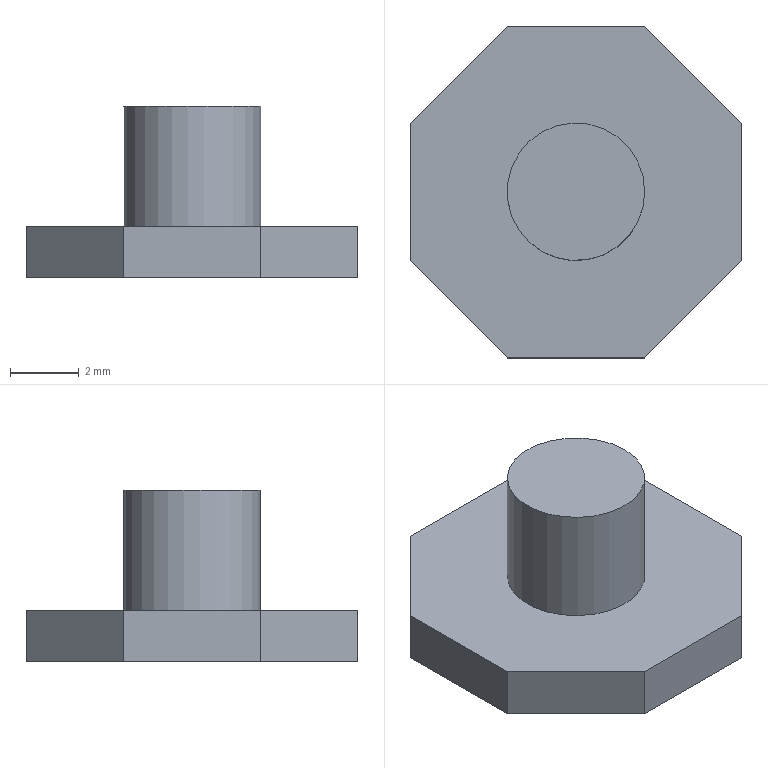Part | NX | features DATUM_CSYS 2, EXTRUDE 2, SKETCH 1 | 1 solid | 12 faces | box 9.657 x 9.657 x 5 mm | volume 159.865 mm3 | plane 11 | cylinder 1 | commonest cylinder face diameters 4 x1
STEP:
#1=CARTESIAN_POINT('',(-4.828,2.,0.));
#2=VERTEX_POINT('',#1);
#3=CARTESIAN_POINT('',(-4.828,-2.,0.));
#4=VERTEX_POINT('',#3);
#5=CARTESIAN_POINT('',(-4.828,2.,0.));
#6=DIRECTION('',(0.,-1.,0.));
#7=VECTOR('',#6,1000.);
#8=LINE('',#5,#7);
#9=EDGE_CURVE('',#2,#4,#8,.T.);
#10=ORIENTED_EDGE('',*,*,#9,.T.);
#11=CARTESIAN_POINT('',(-4.828,-2.,1.5));
#12=VERTEX_POINT('',#11);
#13=CARTESIAN_POINT('',(-4.828,-2.,1.5));
#14=DIRECTION('',(0.,0.,-1.));
#15=VECTOR('',#14,1000.);
#16=LINE('',#13,#15);
#17=EDGE_CURVE('',#12,#4,#16,.T.);
#18=ORIENTED_EDGE('',*,*,#17,.F.);
#19=CARTESIAN_POINT('',(-4.828,2.,1.5));
#20=VERTEX_POINT('',#19);
#21=CARTESIAN_POINT('',(-4.828,2.,1.5));
#22=DIRECTION('',(0.,-1.,0.));
#23=VECTOR('',#22,1000.);
#24=LINE('',#21,#23);
#25=EDGE_CURVE('',#20,#12,#24,.T.);
#26=ORIENTED_EDGE('',*,*,#25,.F.);
#27=CARTESIAN_POINT('',(-4.828,2.,1.5));
#28=DIRECTION('',(0.,0.,-1.));
#29=VECTOR('',#28,1000.);
#30=LINE('',#27,#29);
#31=EDGE_CURVE('',#20,#2,#30,.T.);
#32=ORIENTED_EDGE('',*,*,#31,.T.);
#33=EDGE_LOOP('',(#10,#18,#26,#32));
#34=FACE_BOUND('',#33,.T.);
#35=CARTESIAN_POINT('',(-4.828,2.,1.5));
#36=DIRECTION('',(1.,0.,0.));
#37=DIRECTION('',(0.,0.,-1.));
#38=AXIS2_PLACEMENT_3D('',#35,#36,#37);
#39=PLANE('',#38);
#40=ADVANCED_FACE('',(#34),#39,.F.);
#41=CARTESIAN_POINT('',(-2.,-4.828,0.));
#42=VERTEX_POINT('',#41);
#43=CARTESIAN_POINT('',(-4.828,-2.,0.));
#44=DIRECTION('',(0.7071,-0.7071,0.));
#45=VECTOR('',#44,1000.);
#46=LINE('',#43,#45);
#47=EDGE_CURVE('',#4,#42,#46,.T.);
#48=ORIENTED_EDGE('',*,*,#47,.T.);
#49=CARTESIAN_POINT('',(-2.,-4.828,1.5));
#50=VERTEX_POINT('',#49);
#51=CARTESIAN_POINT('',(-2.,-4.828,1.5));
#52=DIRECTION('',(0.,0.,-1.));
#53=VECTOR('',#52,1000.);
#54=LINE('',#51,#53);
#55=EDGE_CURVE('',#50,#42,#54,.T.);
#56=ORIENTED_EDGE('',*,*,#55,.F.);
#57=CARTESIAN_POINT('',(-4.828,-2.,1.5));
#58=DIRECTION('',(0.7071,-0.7071,0.));
#59=VECTOR('',#58,1000.);
#60=LINE('',#57,#59);
#61=EDGE_CURVE('',#12,#50,#60,.T.);
#62=ORIENTED_EDGE('',*,*,#61,.F.);
#63=ORIENTED_EDGE('',*,*,#17,.T.);
#64=EDGE_LOOP('',(#48,#56,#62,#63));
#65=FACE_BOUND('',#64,.T.);
#66=CARTESIAN_POINT('',(-4.828,-2.,1.5));
#67=DIRECTION('',(0.7071,0.7071,0.));
#68=DIRECTION('',(-0.7071,0.7071,0.));
#69=AXIS2_PLACEMENT_3D('',#66,#67,#68);
#70=PLANE('',#69);
#71=ADVANCED_FACE('',(#65),#70,.F.);
#72=CARTESIAN_POINT('',(2.,-4.828,0.));
#73=VERTEX_POINT('',#72);
#74=CARTESIAN_POINT('',(-2.,-4.828,0.));
#75=DIRECTION('',(1.,0.,0.));
#76=VECTOR('',#75,1000.);
#77=LINE('',#74,#76);
#78=EDGE_CURVE('',#42,#73,#77,.T.);
#79=ORIENTED_EDGE('',*,*,#78,.T.);
#80=CARTESIAN_POINT('',(2.,-4.828,1.5));
#81=VERTEX_POINT('',#80);
#82=CARTESIAN_POINT('',(2.,-4.828,1.5));
#83=DIRECTION('',(0.,0.,-1.));
#84=VECTOR('',#83,1000.);
#85=LINE('',#82,#84);
#86=EDGE_CURVE('',#81,#73,#85,.T.);
#87=ORIENTED_EDGE('',*,*,#86,.F.);
#88=CARTESIAN_POINT('',(-2.,-4.828,1.5));
#89=DIRECTION('',(1.,0.,0.));
#90=VECTOR('',#89,1000.);
#91=LINE('',#88,#90);
#92=EDGE_CURVE('',#50,#81,#91,.T.);
#93=ORIENTED_EDGE('',*,*,#92,.F.);
#94=ORIENTED_EDGE('',*,*,#55,.T.);
#95=EDGE_LOOP('',(#79,#87,#93,#94));
#96=FACE_BOUND('',#95,.T.);
#97=CARTESIAN_POINT('',(-2.,-4.828,1.5));
#98=DIRECTION('',(0.,1.,0.));
#99=DIRECTION('',(-1.,0.,0.));
#100=AXIS2_PLACEMENT_3D('',#97,#98,#99);
#101=PLANE('',#100);
#102=ADVANCED_FACE('',(#96),#101,.F.);
#103=CARTESIAN_POINT('',(4.828,-2.,0.));
#104=VERTEX_POINT('',#103);
#105=CARTESIAN_POINT('',(2.,-4.828,0.));
#106=DIRECTION('',(0.7071,0.7071,0.));
#107=VECTOR('',#106,1000.);
#108=LINE('',#105,#107);
#109=EDGE_CURVE('',#73,#104,#108,.T.);
#110=ORIENTED_EDGE('',*,*,#109,.T.);
#111=CARTESIAN_POINT('',(4.828,-2.,1.5));
#112=VERTEX_POINT('',#111);
#113=CARTESIAN_POINT('',(4.828,-2.,1.5));
#114=DIRECTION('',(0.,0.,-1.));
#115=VECTOR('',#114,1000.);
#116=LINE('',#113,#115);
#117=EDGE_CURVE('',#112,#104,#116,.T.);
#118=ORIENTED_EDGE('',*,*,#117,.F.);
#119=CARTESIAN_POINT('',(2.,-4.828,1.5));
#120=DIRECTION('',(0.7071,0.7071,0.));
#121=VECTOR('',#120,1000.);
#122=LINE('',#119,#121);
#123=EDGE_CURVE('',#81,#112,#122,.T.);
#124=ORIENTED_EDGE('',*,*,#123,.F.);
#125=ORIENTED_EDGE('',*,*,#86,.T.);
#126=EDGE_LOOP('',(#110,#118,#124,#125));
#127=FACE_BOUND('',#126,.T.);
#128=CARTESIAN_POINT('',(2.,-4.828,1.5));
#129=DIRECTION('',(-0.7071,0.7071,0.));
#130=DIRECTION('',(-0.7071,-0.7071,0.));
#131=AXIS2_PLACEMENT_3D('',#128,#129,#130);
#132=PLANE('',#131);
#133=ADVANCED_FACE('',(#127),#132,.F.);
#134=CARTESIAN_POINT('',(4.828,2.,0.));
#135=VERTEX_POINT('',#134);
#136=CARTESIAN_POINT('',(4.828,-2.,0.));
#137=DIRECTION('',(0.,1.,0.));
#138=VECTOR('',#137,1000.);
#139=LINE('',#136,#138);
#140=EDGE_CURVE('',#104,#135,#139,.T.);
#141=ORIENTED_EDGE('',*,*,#140,.T.);
#142=CARTESIAN_POINT('',(4.828,2.,1.5));
#143=VERTEX_POINT('',#142);
#144=CARTESIAN_POINT('',(4.828,2.,1.5));
#145=DIRECTION('',(0.,0.,-1.));
#146=VECTOR('',#145,1000.);
#147=LINE('',#144,#146);
#148=EDGE_CURVE('',#143,#135,#147,.T.);
#149=ORIENTED_EDGE('',*,*,#148,.F.);
#150=CARTESIAN_POINT('',(4.828,-2.,1.5));
#151=DIRECTION('',(0.,1.,0.));
#152=VECTOR('',#151,1000.);
#153=LINE('',#150,#152);
#154=EDGE_CURVE('',#112,#143,#153,.T.);
#155=ORIENTED_EDGE('',*,*,#154,.F.);
#156=ORIENTED_EDGE('',*,*,#117,.T.);
#157=EDGE_LOOP('',(#141,#149,#155,#156));
#158=FACE_BOUND('',#157,.T.);
#159=CARTESIAN_POINT('',(4.828,-2.,1.5));
#160=DIRECTION('',(-1.,0.,0.));
#161=DIRECTION('',(0.,0.,1.));
#162=AXIS2_PLACEMENT_3D('',#159,#160,#161);
#163=PLANE('',#162);
#164=ADVANCED_FACE('',(#158),#163,.F.);
#165=CARTESIAN_POINT('',(2.,4.828,0.));
#166=VERTEX_POINT('',#165);
#167=CARTESIAN_POINT('',(4.828,2.,0.));
#168=DIRECTION('',(-0.7071,0.7071,0.));
#169=VECTOR('',#168,1000.);
#170=LINE('',#167,#169);
#171=EDGE_CURVE('',#135,#166,#170,.T.);
#172=ORIENTED_EDGE('',*,*,#171,.T.);
#173=CARTESIAN_POINT('',(2.,4.828,1.5));
#174=VERTEX_POINT('',#173);
#175=CARTESIAN_POINT('',(2.,4.828,1.5));
#176=DIRECTION('',(0.,0.,-1.));
#177=VECTOR('',#176,1000.);
#178=LINE('',#175,#177);
#179=EDGE_CURVE('',#174,#166,#178,.T.);
#180=ORIENTED_EDGE('',*,*,#179,.F.);
#181=CARTESIAN_POINT('',(4.828,2.,1.5));
#182=DIRECTION('',(-0.7071,0.7071,0.));
#183=VECTOR('',#182,1000.);
#184=LINE('',#181,#183);
#185=EDGE_CURVE('',#143,#174,#184,.T.);
#186=ORIENTED_EDGE('',*,*,#185,.F.);
#187=ORIENTED_EDGE('',*,*,#148,.T.);
#188=EDGE_LOOP('',(#172,#180,#186,#187));
#189=FACE_BOUND('',#188,.T.);
#190=CARTESIAN_POINT('',(4.828,2.,1.5));
#191=DIRECTION('',(-0.7071,-0.7071,0.));
#192=DIRECTION('',(0.7071,-0.7071,0.));
#193=AXIS2_PLACEMENT_3D('',#190,#191,#192);
#194=PLANE('',#193);
#195=ADVANCED_FACE('',(#189),#194,.F.);
#196=CARTESIAN_POINT('',(-2.,4.828,0.));
#197=VERTEX_POINT('',#196);
#198=CARTESIAN_POINT('',(2.,4.828,0.));
#199=DIRECTION('',(-1.,0.,0.));
#200=VECTOR('',#199,1000.);
#201=LINE('',#198,#200);
#202=EDGE_CURVE('',#166,#197,#201,.T.);
#203=ORIENTED_EDGE('',*,*,#202,.T.);
#204=CARTESIAN_POINT('',(-2.,4.828,1.5));
#205=VERTEX_POINT('',#204);
#206=CARTESIAN_POINT('',(-2.,4.828,1.5));
#207=DIRECTION('',(0.,0.,-1.));
#208=VECTOR('',#207,1000.);
#209=LINE('',#206,#208);
#210=EDGE_CURVE('',#205,#197,#209,.T.);
#211=ORIENTED_EDGE('',*,*,#210,.F.);
#212=CARTESIAN_POINT('',(2.,4.828,1.5));
#213=DIRECTION('',(-1.,0.,0.));
#214=VECTOR('',#213,1000.);
#215=LINE('',#212,#214);
#216=EDGE_CURVE('',#174,#205,#215,.T.);
#217=ORIENTED_EDGE('',*,*,#216,.F.);
#218=ORIENTED_EDGE('',*,*,#179,.T.);
#219=EDGE_LOOP('',(#203,#211,#217,#218));
#220=FACE_BOUND('',#219,.T.);
#221=CARTESIAN_POINT('',(2.,4.828,1.5));
#222=DIRECTION('',(0.,-1.,0.));
#223=DIRECTION('',(0.,0.,-1.));
#224=AXIS2_PLACEMENT_3D('',#221,#222,#223);
#225=PLANE('',#224);
#226=ADVANCED_FACE('',(#220),#225,.F.);
#227=CARTESIAN_POINT('',(-2.,4.828,0.));
#228=DIRECTION('',(-0.7071,-0.7071,0.));
#229=VECTOR('',#228,1000.);
#230=LINE('',#227,#229);
#231=EDGE_CURVE('',#197,#2,#230,.T.);
#232=ORIENTED_EDGE('',*,*,#231,.T.);
#233=ORIENTED_EDGE('',*,*,#31,.F.);
#234=CARTESIAN_POINT('',(-2.,4.828,1.5));
#235=DIRECTION('',(-0.7071,-0.7071,0.));
#236=VECTOR('',#235,1000.);
#237=LINE('',#234,#236);
#238=EDGE_CURVE('',#205,#20,#237,.T.);
#239=ORIENTED_EDGE('',*,*,#238,.F.);
#240=ORIENTED_EDGE('',*,*,#210,.T.);
#241=EDGE_LOOP('',(#232,#233,#239,#240));
#242=FACE_BOUND('',#241,.T.);
#243=CARTESIAN_POINT('',(-2.,4.828,1.5));
#244=DIRECTION('',(0.7071,-0.7071,0.));
#245=DIRECTION('',(0.7071,0.7071,0.));
#246=AXIS2_PLACEMENT_3D('',#243,#244,#245);
#247=PLANE('',#246);
#248=ADVANCED_FACE('',(#242),#247,.F.);
#249=CARTESIAN_POINT('',(2.,0.,1.5));
#250=VERTEX_POINT('',#249);
#251=CARTESIAN_POINT('',(0.,0.,1.5));
#252=DIRECTION('',(0.,0.,1.));
#253=DIRECTION('',(1.,0.,0.));
#254=AXIS2_PLACEMENT_3D('',#251,#252,#253);
#255=CIRCLE('',#254,2.);
#256=EDGE_CURVE('',#250,#250,#255,.F.);
#257=ORIENTED_EDGE('',*,*,#256,.T.);
#258=EDGE_LOOP('',(#257));
#259=FACE_BOUND('',#258,.T.);
#260=ORIENTED_EDGE('',*,*,#25,.T.);
#261=ORIENTED_EDGE('',*,*,#61,.T.);
#262=ORIENTED_EDGE('',*,*,#92,.T.);
#263=ORIENTED_EDGE('',*,*,#123,.T.);
#264=ORIENTED_EDGE('',*,*,#154,.T.);
#265=ORIENTED_EDGE('',*,*,#185,.T.);
#266=ORIENTED_EDGE('',*,*,#216,.T.);
#267=ORIENTED_EDGE('',*,*,#238,.T.);
#268=EDGE_LOOP('',(#260,#261,#262,#263,#264,#265,#266,#267));
#269=FACE_BOUND('',#268,.T.);
#270=CARTESIAN_POINT('',(0.,0.,1.5));
#271=DIRECTION('',(0.,0.,1.));
#272=DIRECTION('',(1.,0.,0.));
#273=AXIS2_PLACEMENT_3D('',#270,#271,#272);
#274=PLANE('',#273);
#275=ADVANCED_FACE('',(#259,#269),#274,.T.);
#276=ORIENTED_EDGE('',*,*,#9,.F.);
#277=ORIENTED_EDGE('',*,*,#231,.F.);
#278=ORIENTED_EDGE('',*,*,#202,.F.);
#279=ORIENTED_EDGE('',*,*,#171,.F.);
#280=ORIENTED_EDGE('',*,*,#140,.F.);
#281=ORIENTED_EDGE('',*,*,#109,.F.);
#282=ORIENTED_EDGE('',*,*,#78,.F.);
#283=ORIENTED_EDGE('',*,*,#47,.F.);
#284=EDGE_LOOP('',(#276,#277,#278,#279,#280,#281,#282,#283));
#285=FACE_BOUND('',#284,.T.);
#286=CARTESIAN_POINT('',(0.,0.,0.));
#287=DIRECTION('',(0.,0.,1.));
#288=DIRECTION('',(1.,0.,0.));
#289=AXIS2_PLACEMENT_3D('',#286,#287,#288);
#290=PLANE('',#289);
#291=ADVANCED_FACE('',(#285),#290,.F.);
#292=ORIENTED_EDGE('',*,*,#256,.F.);
#293=EDGE_LOOP('',(#292));
#294=FACE_BOUND('',#293,.T.);
#295=CARTESIAN_POINT('',(2.,0.,5.));
#296=VERTEX_POINT('',#295);
#297=CARTESIAN_POINT('',(0.,0.,5.));
#298=DIRECTION('',(0.,0.,1.));
#299=DIRECTION('',(1.,0.,0.));
#300=AXIS2_PLACEMENT_3D('',#297,#298,#299);
#301=CIRCLE('',#300,2.);
#302=EDGE_CURVE('',#296,#296,#301,.T.);
#303=ORIENTED_EDGE('',*,*,#302,.F.);
#304=EDGE_LOOP('',(#303));
#305=FACE_BOUND('',#304,.T.);
#306=CARTESIAN_POINT('',(0.,0.,5.));
#307=DIRECTION('',(0.,0.,-1.));
#308=DIRECTION('',(-1.,0.,0.));
#309=AXIS2_PLACEMENT_3D('',#306,#307,#308);
#310=CYLINDRICAL_SURFACE('',#309,2.);
#311=ADVANCED_FACE('',(#294,#305),#310,.T.);
#312=ORIENTED_EDGE('',*,*,#302,.T.);
#313=EDGE_LOOP('',(#312));
#314=FACE_BOUND('',#313,.T.);
#315=CARTESIAN_POINT('',(0.,0.,5.));
#316=DIRECTION('',(0.,0.,1.));
#317=DIRECTION('',(1.,0.,0.));
#318=AXIS2_PLACEMENT_3D('',#315,#316,#317);
#319=PLANE('',#318);
#320=ADVANCED_FACE('',(#314),#319,.T.);
#321=CLOSED_SHELL('',(#40,#71,#102,#133,#164,#195,#226,#248,#275,#291,#311,#320));
#322=MANIFOLD_SOLID_BREP('',#321);
#323=(LENGTH_UNIT()NAMED_UNIT(*)SI_UNIT(.MILLI.,.METRE.));
#324=UNCERTAINTY_MEASURE_WITH_UNIT(LENGTH_MEASURE(0.00001),#323,'','');
#325=(NAMED_UNIT(*)PLANE_ANGLE_UNIT()SI_UNIT($,.RADIAN.));
#326=(NAMED_UNIT(*)SI_UNIT($,.STERADIAN.)SOLID_ANGLE_UNIT());
#327=(GEOMETRIC_REPRESENTATION_CONTEXT(3)GLOBAL_UNCERTAINTY_ASSIGNED_CONTEXT((#324))GLOBAL_UNIT_ASSIGNED_CONTEXT((#323,#325,#326))REPRESENTATION_CONTEXT('',''));
#328=ADVANCED_BREP_SHAPE_REPRESENTATION('',(#322),#327);